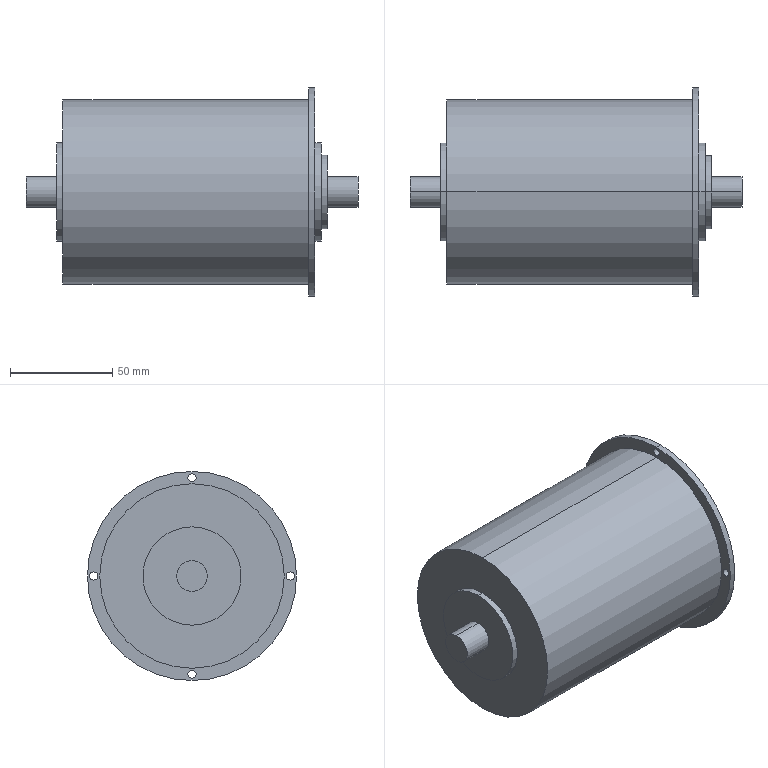Part | NX | features BREP 1 | 1 solid | 30 faces | box 162 x 102 x 102 mm | volume 806982 mm3 | cylinder 22 | plane 8 | commonest cylinder face diameters 4 x8 15 x4 48 x4 36 x2 90 x2 102 x2
STEP:
#1=CARTESIAN_POINT('',(141.,0.,-46.));
#2=VERTEX_POINT('',#1);
#3=CARTESIAN_POINT('',(141.,0.,-50.));
#4=VERTEX_POINT('',#3);
#5=CARTESIAN_POINT('',(141.,0.,-48.));
#6=DIRECTION('',(1.,0.,0.));
#7=DIRECTION('',(0.,0.,1.));
#8=AXIS2_PLACEMENT_3D('',#5,#6,#7);
#9=CIRCLE('',#8,2.);
#10=EDGE_CURVE('',#2,#4,#9,.T.);
#11=ORIENTED_EDGE('',*,*,#10,.T.);
#12=CARTESIAN_POINT('',(138.,0.,-50.));
#13=VERTEX_POINT('',#12);
#14=CARTESIAN_POINT('',(162.001,0.,-50.));
#15=DIRECTION('',(-1.,0.,0.));
#16=VECTOR('',#15,1000.);
#17=LINE('',#14,#16);
#18=EDGE_CURVE('',#4,#13,#17,.T.);
#19=ORIENTED_EDGE('',*,*,#18,.T.);
#20=CARTESIAN_POINT('',(138.,0.,-46.));
#21=VERTEX_POINT('',#20);
#22=CARTESIAN_POINT('',(138.,0.,-48.));
#23=DIRECTION('',(-1.,0.,0.));
#24=DIRECTION('',(0.,0.,1.));
#25=AXIS2_PLACEMENT_3D('',#22,#23,#24);
#26=CIRCLE('',#25,2.);
#27=EDGE_CURVE('',#13,#21,#26,.T.);
#28=ORIENTED_EDGE('',*,*,#27,.T.);
#29=CARTESIAN_POINT('',(162.001,0.,-46.));
#30=DIRECTION('',(-1.,0.,0.));
#31=VECTOR('',#30,1000.);
#32=LINE('',#29,#31);
#33=EDGE_CURVE('',#2,#21,#32,.T.);
#34=ORIENTED_EDGE('',*,*,#33,.F.);
#35=EDGE_LOOP('',(#11,#19,#28,#34));
#36=FACE_BOUND('',#35,.T.);
#37=CARTESIAN_POINT('',(162.001,0.,-48.));
#38=DIRECTION('',(-1.,0.,0.));
#39=DIRECTION('',(0.,0.,-1.));
#40=AXIS2_PLACEMENT_3D('',#37,#38,#39);
#41=CYLINDRICAL_SURFACE('',#40,2.);
#42=ADVANCED_FACE('',(#36),#41,.F.);
#43=CARTESIAN_POINT('',(141.,-48.,2.));
#44=VERTEX_POINT('',#43);
#45=CARTESIAN_POINT('',(141.,-48.,-2.));
#46=VERTEX_POINT('',#45);
#47=CARTESIAN_POINT('',(141.,-48.,0.));
#48=DIRECTION('',(1.,0.,0.));
#49=DIRECTION('',(0.,0.,1.));
#50=AXIS2_PLACEMENT_3D('',#47,#48,#49);
#51=CIRCLE('',#50,2.);
#52=EDGE_CURVE('',#44,#46,#51,.T.);
#53=ORIENTED_EDGE('',*,*,#52,.T.);
#54=CARTESIAN_POINT('',(138.,-48.,-2.));
#55=VERTEX_POINT('',#54);
#56=CARTESIAN_POINT('',(162.001,-48.,-2.));
#57=DIRECTION('',(-1.,0.,0.));
#58=VECTOR('',#57,1000.);
#59=LINE('',#56,#58);
#60=EDGE_CURVE('',#46,#55,#59,.T.);
#61=ORIENTED_EDGE('',*,*,#60,.T.);
#62=CARTESIAN_POINT('',(138.,-48.,2.));
#63=VERTEX_POINT('',#62);
#64=CARTESIAN_POINT('',(138.,-48.,0.));
#65=DIRECTION('',(-1.,0.,0.));
#66=DIRECTION('',(0.,0.,1.));
#67=AXIS2_PLACEMENT_3D('',#64,#65,#66);
#68=CIRCLE('',#67,2.);
#69=EDGE_CURVE('',#55,#63,#68,.T.);
#70=ORIENTED_EDGE('',*,*,#69,.T.);
#71=CARTESIAN_POINT('',(162.001,-48.,2.));
#72=DIRECTION('',(-1.,0.,0.));
#73=VECTOR('',#72,1000.);
#74=LINE('',#71,#73);
#75=EDGE_CURVE('',#44,#63,#74,.T.);
#76=ORIENTED_EDGE('',*,*,#75,.F.);
#77=EDGE_LOOP('',(#53,#61,#70,#76));
#78=FACE_BOUND('',#77,.T.);
#79=CARTESIAN_POINT('',(162.001,-48.,0.));
#80=DIRECTION('',(-1.,0.,0.));
#81=DIRECTION('',(0.,0.,-1.));
#82=AXIS2_PLACEMENT_3D('',#79,#80,#81);
#83=CYLINDRICAL_SURFACE('',#82,2.);
#84=ADVANCED_FACE('',(#78),#83,.F.);
#85=CARTESIAN_POINT('',(141.,0.,50.));
#86=VERTEX_POINT('',#85);
#87=CARTESIAN_POINT('',(141.,0.,46.));
#88=VERTEX_POINT('',#87);
#89=CARTESIAN_POINT('',(141.,0.,48.));
#90=DIRECTION('',(1.,0.,0.));
#91=DIRECTION('',(0.,0.,1.));
#92=AXIS2_PLACEMENT_3D('',#89,#90,#91);
#93=CIRCLE('',#92,2.);
#94=EDGE_CURVE('',#86,#88,#93,.T.);
#95=ORIENTED_EDGE('',*,*,#94,.T.);
#96=CARTESIAN_POINT('',(138.,0.,46.));
#97=VERTEX_POINT('',#96);
#98=CARTESIAN_POINT('',(162.001,0.,46.));
#99=DIRECTION('',(-1.,0.,0.));
#100=VECTOR('',#99,1000.);
#101=LINE('',#98,#100);
#102=EDGE_CURVE('',#88,#97,#101,.T.);
#103=ORIENTED_EDGE('',*,*,#102,.T.);
#104=CARTESIAN_POINT('',(138.,0.,50.));
#105=VERTEX_POINT('',#104);
#106=CARTESIAN_POINT('',(138.,0.,48.));
#107=DIRECTION('',(-1.,0.,0.));
#108=DIRECTION('',(0.,0.,1.));
#109=AXIS2_PLACEMENT_3D('',#106,#107,#108);
#110=CIRCLE('',#109,2.);
#111=EDGE_CURVE('',#97,#105,#110,.T.);
#112=ORIENTED_EDGE('',*,*,#111,.T.);
#113=CARTESIAN_POINT('',(162.001,0.,50.));
#114=DIRECTION('',(-1.,0.,0.));
#115=VECTOR('',#114,1000.);
#116=LINE('',#113,#115);
#117=EDGE_CURVE('',#86,#105,#116,.T.);
#118=ORIENTED_EDGE('',*,*,#117,.F.);
#119=EDGE_LOOP('',(#95,#103,#112,#118));
#120=FACE_BOUND('',#119,.T.);
#121=CARTESIAN_POINT('',(162.001,0.,48.));
#122=DIRECTION('',(-1.,0.,0.));
#123=DIRECTION('',(0.,0.,-1.));
#124=AXIS2_PLACEMENT_3D('',#121,#122,#123);
#125=CYLINDRICAL_SURFACE('',#124,2.);
#126=ADVANCED_FACE('',(#120),#125,.F.);
#127=CARTESIAN_POINT('',(141.,48.,2.));
#128=VERTEX_POINT('',#127);
#129=CARTESIAN_POINT('',(141.,48.,-2.));
#130=VERTEX_POINT('',#129);
#131=CARTESIAN_POINT('',(141.,48.,0.));
#132=DIRECTION('',(1.,0.,0.));
#133=DIRECTION('',(0.,0.,1.));
#134=AXIS2_PLACEMENT_3D('',#131,#132,#133);
#135=CIRCLE('',#134,2.);
#136=EDGE_CURVE('',#128,#130,#135,.T.);
#137=ORIENTED_EDGE('',*,*,#136,.T.);
#138=CARTESIAN_POINT('',(138.,48.,-2.));
#139=VERTEX_POINT('',#138);
#140=CARTESIAN_POINT('',(162.001,48.,-2.));
#141=DIRECTION('',(-1.,0.,0.));
#142=VECTOR('',#141,1000.);
#143=LINE('',#140,#142);
#144=EDGE_CURVE('',#130,#139,#143,.T.);
#145=ORIENTED_EDGE('',*,*,#144,.T.);
#146=CARTESIAN_POINT('',(138.,48.,2.));
#147=VERTEX_POINT('',#146);
#148=CARTESIAN_POINT('',(138.,48.,0.));
#149=DIRECTION('',(-1.,0.,0.));
#150=DIRECTION('',(0.,0.,1.));
#151=AXIS2_PLACEMENT_3D('',#148,#149,#150);
#152=CIRCLE('',#151,2.);
#153=EDGE_CURVE('',#139,#147,#152,.T.);
#154=ORIENTED_EDGE('',*,*,#153,.T.);
#155=CARTESIAN_POINT('',(162.001,48.,2.));
#156=DIRECTION('',(-1.,0.,0.));
#157=VECTOR('',#156,1000.);
#158=LINE('',#155,#157);
#159=EDGE_CURVE('',#128,#147,#158,.T.);
#160=ORIENTED_EDGE('',*,*,#159,.F.);
#161=EDGE_LOOP('',(#137,#145,#154,#160));
#162=FACE_BOUND('',#161,.T.);
#163=CARTESIAN_POINT('',(162.001,48.,0.));
#164=DIRECTION('',(-1.,0.,0.));
#165=DIRECTION('',(0.,0.,-1.));
#166=AXIS2_PLACEMENT_3D('',#163,#164,#165);
#167=CYLINDRICAL_SURFACE('',#166,2.);
#168=ADVANCED_FACE('',(#162),#167,.F.);
#169=CARTESIAN_POINT('',(162.,0.,7.5));
#170=VERTEX_POINT('',#169);
#171=CARTESIAN_POINT('',(162.,0.,-7.5));
#172=VERTEX_POINT('',#171);
#173=CARTESIAN_POINT('',(162.,0.,0.));
#174=DIRECTION('',(-1.,0.,0.));
#175=DIRECTION('',(0.,0.,1.));
#176=AXIS2_PLACEMENT_3D('',#173,#174,#175);
#177=CIRCLE('',#176,7.5);
#178=EDGE_CURVE('',#170,#172,#177,.T.);
#179=ORIENTED_EDGE('',*,*,#178,.T.);
#180=CARTESIAN_POINT('',(147.,0.,-7.5));
#181=VERTEX_POINT('',#180);
#182=CARTESIAN_POINT('',(0.,0.,-7.5));
#183=DIRECTION('',(-1.,0.,0.));
#184=VECTOR('',#183,1000.);
#185=LINE('',#182,#184);
#186=EDGE_CURVE('',#172,#181,#185,.T.);
#187=ORIENTED_EDGE('',*,*,#186,.T.);
#188=CARTESIAN_POINT('',(147.,0.,7.5));
#189=VERTEX_POINT('',#188);
#190=CARTESIAN_POINT('',(147.,0.,0.));
#191=DIRECTION('',(-1.,0.,0.));
#192=DIRECTION('',(0.,0.,1.));
#193=AXIS2_PLACEMENT_3D('',#190,#191,#192);
#194=CIRCLE('',#193,7.5);
#195=EDGE_CURVE('',#189,#181,#194,.T.);
#196=ORIENTED_EDGE('',*,*,#195,.F.);
#197=CARTESIAN_POINT('',(0.,0.,7.5));
#198=DIRECTION('',(-1.,0.,0.));
#199=VECTOR('',#198,1000.);
#200=LINE('',#197,#199);
#201=EDGE_CURVE('',#170,#189,#200,.T.);
#202=ORIENTED_EDGE('',*,*,#201,.F.);
#203=EDGE_LOOP('',(#179,#187,#196,#202));
#204=FACE_BOUND('',#203,.T.);
#205=CARTESIAN_POINT('',(0.,0.,0.));
#206=DIRECTION('',(-1.,0.,0.));
#207=DIRECTION('',(0.,0.,-1.));
#208=AXIS2_PLACEMENT_3D('',#205,#206,#207);
#209=CYLINDRICAL_SURFACE('',#208,7.5);
#210=ADVANCED_FACE('',(#204),#209,.T.);
#211=CARTESIAN_POINT('',(147.,0.,18.));
#212=VERTEX_POINT('',#211);
#213=CARTESIAN_POINT('',(147.,0.,-18.));
#214=VERTEX_POINT('',#213);
#215=CARTESIAN_POINT('',(147.,0.,0.));
#216=DIRECTION('',(-1.,0.,0.));
#217=DIRECTION('',(0.,0.,1.));
#218=AXIS2_PLACEMENT_3D('',#215,#216,#217);
#219=CIRCLE('',#218,18.);
#220=EDGE_CURVE('',#212,#214,#219,.T.);
#221=ORIENTED_EDGE('',*,*,#220,.T.);
#222=CARTESIAN_POINT('',(144.,0.,-18.));
#223=VERTEX_POINT('',#222);
#224=CARTESIAN_POINT('',(0.,0.,-18.));
#225=DIRECTION('',(-1.,0.,0.));
#226=VECTOR('',#225,1000.);
#227=LINE('',#224,#226);
#228=EDGE_CURVE('',#214,#223,#227,.T.);
#229=ORIENTED_EDGE('',*,*,#228,.T.);
#230=CARTESIAN_POINT('',(144.,0.,18.));
#231=VERTEX_POINT('',#230);
#232=CARTESIAN_POINT('',(144.,0.,0.));
#233=DIRECTION('',(-1.,0.,0.));
#234=DIRECTION('',(0.,0.,1.));
#235=AXIS2_PLACEMENT_3D('',#232,#233,#234);
#236=CIRCLE('',#235,18.);
#237=EDGE_CURVE('',#231,#223,#236,.T.);
#238=ORIENTED_EDGE('',*,*,#237,.F.);
#239=CARTESIAN_POINT('',(0.,0.,18.));
#240=DIRECTION('',(-1.,0.,0.));
#241=VECTOR('',#240,1000.);
#242=LINE('',#239,#241);
#243=EDGE_CURVE('',#212,#231,#242,.T.);
#244=ORIENTED_EDGE('',*,*,#243,.F.);
#245=EDGE_LOOP('',(#221,#229,#238,#244));
#246=FACE_BOUND('',#245,.T.);
#247=CARTESIAN_POINT('',(0.,0.,0.));
#248=DIRECTION('',(-1.,0.,0.));
#249=DIRECTION('',(0.,0.,-1.));
#250=AXIS2_PLACEMENT_3D('',#247,#248,#249);
#251=CYLINDRICAL_SURFACE('',#250,18.);
#252=ADVANCED_FACE('',(#246),#251,.T.);
#253=CARTESIAN_POINT('',(144.,0.,24.));
#254=VERTEX_POINT('',#253);
#255=CARTESIAN_POINT('',(144.,0.,-24.));
#256=VERTEX_POINT('',#255);
#257=CARTESIAN_POINT('',(144.,0.,0.));
#258=DIRECTION('',(-1.,0.,0.));
#259=DIRECTION('',(0.,0.,1.));
#260=AXIS2_PLACEMENT_3D('',#257,#258,#259);
#261=CIRCLE('',#260,24.);
#262=EDGE_CURVE('',#254,#256,#261,.T.);
#263=ORIENTED_EDGE('',*,*,#262,.T.);
#264=CARTESIAN_POINT('',(141.,0.,-24.));
#265=VERTEX_POINT('',#264);
#266=CARTESIAN_POINT('',(0.,0.,-24.));
#267=DIRECTION('',(-1.,0.,0.));
#268=VECTOR('',#267,1000.);
#269=LINE('',#266,#268);
#270=EDGE_CURVE('',#256,#265,#269,.T.);
#271=ORIENTED_EDGE('',*,*,#270,.T.);
#272=CARTESIAN_POINT('',(141.,0.,24.));
#273=VERTEX_POINT('',#272);
#274=CARTESIAN_POINT('',(141.,0.,0.));
#275=DIRECTION('',(-1.,0.,0.));
#276=DIRECTION('',(0.,0.,1.));
#277=AXIS2_PLACEMENT_3D('',#274,#275,#276);
#278=CIRCLE('',#277,24.);
#279=EDGE_CURVE('',#273,#265,#278,.T.);
#280=ORIENTED_EDGE('',*,*,#279,.F.);
#281=CARTESIAN_POINT('',(0.,0.,24.));
#282=DIRECTION('',(-1.,0.,0.));
#283=VECTOR('',#282,1000.);
#284=LINE('',#281,#283);
#285=EDGE_CURVE('',#254,#273,#284,.T.);
#286=ORIENTED_EDGE('',*,*,#285,.F.);
#287=EDGE_LOOP('',(#263,#271,#280,#286));
#288=FACE_BOUND('',#287,.T.);
#289=CARTESIAN_POINT('',(0.,0.,0.));
#290=DIRECTION('',(-1.,0.,0.));
#291=DIRECTION('',(0.,0.,-1.));
#292=AXIS2_PLACEMENT_3D('',#289,#290,#291);
#293=CYLINDRICAL_SURFACE('',#292,24.);
#294=ADVANCED_FACE('',(#288),#293,.T.);
#295=CARTESIAN_POINT('',(141.,0.,51.));
#296=VERTEX_POINT('',#295);
#297=CARTESIAN_POINT('',(141.,0.,-51.));
#298=VERTEX_POINT('',#297);
#299=CARTESIAN_POINT('',(141.,0.,0.));
#300=DIRECTION('',(-1.,0.,0.));
#301=DIRECTION('',(0.,0.,1.));
#302=AXIS2_PLACEMENT_3D('',#299,#300,#301);
#303=CIRCLE('',#302,51.);
#304=EDGE_CURVE('',#296,#298,#303,.T.);
#305=ORIENTED_EDGE('',*,*,#304,.T.);
#306=CARTESIAN_POINT('',(138.,0.,-51.));
#307=VERTEX_POINT('',#306);
#308=CARTESIAN_POINT('',(0.,0.,-51.));
#309=DIRECTION('',(-1.,0.,0.));
#310=VECTOR('',#309,1000.);
#311=LINE('',#308,#310);
#312=EDGE_CURVE('',#298,#307,#311,.T.);
#313=ORIENTED_EDGE('',*,*,#312,.T.);
#314=CARTESIAN_POINT('',(138.,0.,51.));
#315=VERTEX_POINT('',#314);
#316=CARTESIAN_POINT('',(138.,0.,0.));
#317=DIRECTION('',(-1.,0.,0.));
#318=DIRECTION('',(0.,0.,1.));
#319=AXIS2_PLACEMENT_3D('',#316,#317,#318);
#320=CIRCLE('',#319,51.);
#321=EDGE_CURVE('',#315,#307,#320,.T.);
#322=ORIENTED_EDGE('',*,*,#321,.F.);
#323=CARTESIAN_POINT('',(0.,0.,51.));
#324=DIRECTION('',(-1.,0.,0.));
#325=VECTOR('',#324,1000.);
#326=LINE('',#323,#325);
#327=EDGE_CURVE('',#296,#315,#326,.T.);
#328=ORIENTED_EDGE('',*,*,#327,.F.);
#329=EDGE_LOOP('',(#305,#313,#322,#328));
#330=FACE_BOUND('',#329,.T.);
#331=CARTESIAN_POINT('',(0.,0.,0.));
#332=DIRECTION('',(-1.,0.,0.));
#333=DIRECTION('',(0.,0.,-1.));
#334=AXIS2_PLACEMENT_3D('',#331,#332,#333);
#335=CYLINDRICAL_SURFACE('',#334,51.);
#336=ADVANCED_FACE('',(#330),#335,.T.);
#337=CARTESIAN_POINT('',(138.,0.,45.));
#338=VERTEX_POINT('',#337);
#339=CARTESIAN_POINT('',(138.,0.,-45.));
#340=VERTEX_POINT('',#339);
#341=CARTESIAN_POINT('',(138.,0.,0.));
#342=DIRECTION('',(-1.,0.,0.));
#343=DIRECTION('',(0.,0.,1.));
#344=AXIS2_PLACEMENT_3D('',#341,#342,#343);
#345=CIRCLE('',#344,45.);
#346=EDGE_CURVE('',#338,#340,#345,.T.);
#347=ORIENTED_EDGE('',*,*,#346,.T.);
#348=CARTESIAN_POINT('',(18.,0.,-45.));
#349=VERTEX_POINT('',#348);
#350=CARTESIAN_POINT('',(0.,0.,-45.));
#351=DIRECTION('',(-1.,0.,0.));
#352=VECTOR('',#351,1000.);
#353=LINE('',#350,#352);
#354=EDGE_CURVE('',#340,#349,#353,.T.);
#355=ORIENTED_EDGE('',*,*,#354,.T.);
#356=CARTESIAN_POINT('',(18.,0.,45.));
#357=VERTEX_POINT('',#356);
#358=CARTESIAN_POINT('',(18.,0.,0.));
#359=DIRECTION('',(-1.,0.,0.));
#360=DIRECTION('',(0.,0.,1.));
#361=AXIS2_PLACEMENT_3D('',#358,#359,#360);
#362=CIRCLE('',#361,45.);
#363=EDGE_CURVE('',#357,#349,#362,.T.);
#364=ORIENTED_EDGE('',*,*,#363,.F.);
#365=CARTESIAN_POINT('',(0.,0.,45.));
#366=DIRECTION('',(-1.,0.,0.));
#367=VECTOR('',#366,1000.);
#368=LINE('',#365,#367);
#369=EDGE_CURVE('',#338,#357,#368,.T.);
#370=ORIENTED_EDGE('',*,*,#369,.F.);
#371=EDGE_LOOP('',(#347,#355,#364,#370));
#372=FACE_BOUND('',#371,.T.);
#373=CARTESIAN_POINT('',(0.,0.,0.));
#374=DIRECTION('',(-1.,0.,0.));
#375=DIRECTION('',(0.,0.,-1.));
#376=AXIS2_PLACEMENT_3D('',#373,#374,#375);
#377=CYLINDRICAL_SURFACE('',#376,45.);
#378=ADVANCED_FACE('',(#372),#377,.T.);
#379=CARTESIAN_POINT('',(18.,0.,24.));
#380=VERTEX_POINT('',#379);
#381=CARTESIAN_POINT('',(18.,0.,-24.));
#382=VERTEX_POINT('',#381);
#383=CARTESIAN_POINT('',(18.,0.,0.));
#384=DIRECTION('',(-1.,0.,0.));
#385=DIRECTION('',(0.,0.,1.));
#386=AXIS2_PLACEMENT_3D('',#383,#384,#385);
#387=CIRCLE('',#386,24.);
#388=EDGE_CURVE('',#380,#382,#387,.T.);
#389=ORIENTED_EDGE('',*,*,#388,.T.);
#390=CARTESIAN_POINT('',(15.,0.,-24.));
#391=VERTEX_POINT('',#390);
#392=CARTESIAN_POINT('',(0.,0.,-24.));
#393=DIRECTION('',(-1.,0.,0.));
#394=VECTOR('',#393,1000.);
#395=LINE('',#392,#394);
#396=EDGE_CURVE('',#382,#391,#395,.T.);
#397=ORIENTED_EDGE('',*,*,#396,.T.);
#398=CARTESIAN_POINT('',(15.,0.,24.));
#399=VERTEX_POINT('',#398);
#400=CARTESIAN_POINT('',(15.,0.,0.));
#401=DIRECTION('',(-1.,0.,0.));
#402=DIRECTION('',(0.,0.,1.));
#403=AXIS2_PLACEMENT_3D('',#400,#401,#402);
#404=CIRCLE('',#403,24.);
#405=EDGE_CURVE('',#399,#391,#404,.T.);
#406=ORIENTED_EDGE('',*,*,#405,.F.);
#407=CARTESIAN_POINT('',(0.,0.,24.));
#408=DIRECTION('',(-1.,0.,0.));
#409=VECTOR('',#408,1000.);
#410=LINE('',#407,#409);
#411=EDGE_CURVE('',#380,#399,#410,.T.);
#412=ORIENTED_EDGE('',*,*,#411,.F.);
#413=EDGE_LOOP('',(#389,#397,#406,#412));
#414=FACE_BOUND('',#413,.T.);
#415=CARTESIAN_POINT('',(0.,0.,0.));
#416=DIRECTION('',(-1.,0.,0.));
#417=DIRECTION('',(0.,0.,-1.));
#418=AXIS2_PLACEMENT_3D('',#415,#416,#417);
#419=CYLINDRICAL_SURFACE('',#418,24.);
#420=ADVANCED_FACE('',(#414),#419,.T.);
#421=CARTESIAN_POINT('',(15.,0.,7.5));
#422=VERTEX_POINT('',#421);
#423=CARTESIAN_POINT('',(15.,0.,-7.5));
#424=VERTEX_POINT('',#423);
#425=CARTESIAN_POINT('',(15.,0.,0.));
#426=DIRECTION('',(-1.,0.,0.));
#427=DIRECTION('',(0.,0.,1.));
#428=AXIS2_PLACEMENT_3D('',#425,#426,#427);
#429=CIRCLE('',#428,7.5);
#430=EDGE_CURVE('',#422,#424,#429,.T.);
#431=ORIENTED_EDGE('',*,*,#430,.T.);
#432=CARTESIAN_POINT('',(0.,0.,-7.5));
#433=VERTEX_POINT('',#432);
#434=CARTESIAN_POINT('',(0.,0.,-7.5));
#435=DIRECTION('',(-1.,0.,0.));
#436=VECTOR('',#435,1000.);
#437=LINE('',#434,#436);
#438=EDGE_CURVE('',#424,#433,#437,.T.);
#439=ORIENTED_EDGE('',*,*,#438,.T.);
#440=CARTESIAN_POINT('',(0.,0.,7.5));
#441=VERTEX_POINT('',#440);
#442=CARTESIAN_POINT('',(0.,0.,0.));
#443=DIRECTION('',(-1.,0.,0.));
#444=DIRECTION('',(0.,0.,1.));
#445=AXIS2_PLACEMENT_3D('',#442,#443,#444);
#446=CIRCLE('',#445,7.5);
#447=EDGE_CURVE('',#441,#433,#446,.T.);
#448=ORIENTED_EDGE('',*,*,#447,.F.);
#449=CARTESIAN_POINT('',(0.,0.,7.5));
#450=DIRECTION('',(-1.,0.,0.));
#451=VECTOR('',#450,1000.);
#452=LINE('',#449,#451);
#453=EDGE_CURVE('',#422,#441,#452,.T.);
#454=ORIENTED_EDGE('',*,*,#453,.F.);
#455=EDGE_LOOP('',(#431,#439,#448,#454));
#456=FACE_BOUND('',#455,.T.);
#457=CARTESIAN_POINT('',(0.,0.,0.));
#458=DIRECTION('',(-1.,0.,0.));
#459=DIRECTION('',(0.,0.,-1.));
#460=AXIS2_PLACEMENT_3D('',#457,#458,#459);
#461=CYLINDRICAL_SURFACE('',#460,7.5);
#462=ADVANCED_FACE('',(#456),#461,.T.);
#463=ORIENTED_EDGE('',*,*,#447,.T.);
#464=CARTESIAN_POINT('',(0.,0.,0.));
#465=DIRECTION('',(-1.,0.,0.));
#466=DIRECTION('',(0.,0.,1.));
#467=AXIS2_PLACEMENT_3D('',#464,#465,#466);
#468=CIRCLE('',#467,7.5);
#469=EDGE_CURVE('',#433,#441,#468,.T.);
#470=ORIENTED_EDGE('',*,*,#469,.T.);
#471=EDGE_LOOP('',(#463,#470));
#472=FACE_BOUND('',#471,.T.);
#473=CARTESIAN_POINT('',(0.,0.,0.));
#474=DIRECTION('',(1.,0.,0.));
#475=DIRECTION('',(0.,-1.,0.));
#476=AXIS2_PLACEMENT_3D('',#473,#474,#475);
#477=PLANE('',#476);
#478=ADVANCED_FACE('',(#472),#477,.F.);
#479=ORIENTED_EDGE('',*,*,#438,.F.);
#480=CARTESIAN_POINT('',(15.,0.,0.));
#481=DIRECTION('',(-1.,0.,0.));
#482=DIRECTION('',(0.,0.,1.));
#483=AXIS2_PLACEMENT_3D('',#480,#481,#482);
#484=CIRCLE('',#483,7.5);
#485=EDGE_CURVE('',#424,#422,#484,.T.);
#486=ORIENTED_EDGE('',*,*,#485,.T.);
#487=ORIENTED_EDGE('',*,*,#453,.T.);
#488=ORIENTED_EDGE('',*,*,#469,.F.);
#489=EDGE_LOOP('',(#479,#486,#487,#488));
#490=FACE_BOUND('',#489,.T.);
#491=CARTESIAN_POINT('',(0.,0.,0.));
#492=DIRECTION('',(-1.,0.,0.));
#493=DIRECTION('',(0.,0.,-1.));
#494=AXIS2_PLACEMENT_3D('',#491,#492,#493);
#495=CYLINDRICAL_SURFACE('',#494,7.5);
#496=ADVANCED_FACE('',(#490),#495,.T.);
#497=ORIENTED_EDGE('',*,*,#405,.T.);
#498=CARTESIAN_POINT('',(15.,0.,0.));
#499=DIRECTION('',(-1.,0.,0.));
#500=DIRECTION('',(0.,0.,1.));
#501=AXIS2_PLACEMENT_3D('',#498,#499,#500);
#502=CIRCLE('',#501,24.);
#503=EDGE_CURVE('',#391,#399,#502,.T.);
#504=ORIENTED_EDGE('',*,*,#503,.T.);
#505=EDGE_LOOP('',(#497,#504));
#506=FACE_BOUND('',#505,.T.);
#507=ORIENTED_EDGE('',*,*,#430,.F.);
#508=ORIENTED_EDGE('',*,*,#485,.F.);
#509=EDGE_LOOP('',(#507,#508));
#510=FACE_BOUND('',#509,.T.);
#511=CARTESIAN_POINT('',(15.,7.5,0.));
#512=DIRECTION('',(1.,0.,0.));
#513=DIRECTION('',(0.,-1.,0.));
#514=AXIS2_PLACEMENT_3D('',#511,#512,#513);
#515=PLANE('',#514);
#516=ADVANCED_FACE('',(#506,#510),#515,.F.);
#517=ORIENTED_EDGE('',*,*,#396,.F.);
#518=CARTESIAN_POINT('',(18.,0.,0.));
#519=DIRECTION('',(-1.,0.,0.));
#520=DIRECTION('',(0.,0.,1.));
#521=AXIS2_PLACEMENT_3D('',#518,#519,#520);
#522=CIRCLE('',#521,24.);
#523=EDGE_CURVE('',#382,#380,#522,.T.);
#524=ORIENTED_EDGE('',*,*,#523,.T.);
#525=ORIENTED_EDGE('',*,*,#411,.T.);
#526=ORIENTED_EDGE('',*,*,#503,.F.);
#527=EDGE_LOOP('',(#517,#524,#525,#526));
#528=FACE_BOUND('',#527,.T.);
#529=CARTESIAN_POINT('',(0.,0.,0.));
#530=DIRECTION('',(-1.,0.,0.));
#531=DIRECTION('',(0.,0.,-1.));
#532=AXIS2_PLACEMENT_3D('',#529,#530,#531);
#533=CYLINDRICAL_SURFACE('',#532,24.);
#534=ADVANCED_FACE('',(#528),#533,.T.);
#535=ORIENTED_EDGE('',*,*,#363,.T.);
#536=CARTESIAN_POINT('',(18.,0.,0.));
#537=DIRECTION('',(-1.,0.,0.));
#538=DIRECTION('',(0.,0.,1.));
#539=AXIS2_PLACEMENT_3D('',#536,#537,#538);
#540=CIRCLE('',#539,45.);
#541=EDGE_CURVE('',#349,#357,#540,.T.);
#542=ORIENTED_EDGE('',*,*,#541,.T.);
#543=EDGE_LOOP('',(#535,#542));
#544=FACE_BOUND('',#543,.T.);
#545=ORIENTED_EDGE('',*,*,#388,.F.);
#546=ORIENTED_EDGE('',*,*,#523,.F.);
#547=EDGE_LOOP('',(#545,#546));
#548=FACE_BOUND('',#547,.T.);
#549=CARTESIAN_POINT('',(18.,24.,0.));
#550=DIRECTION('',(1.,0.,0.));
#551=DIRECTION('',(0.,-1.,0.));
#552=AXIS2_PLACEMENT_3D('',#549,#550,#551);
#553=PLANE('',#552);
#554=ADVANCED_FACE('',(#544,#548),#553,.F.);
#555=ORIENTED_EDGE('',*,*,#354,.F.);
#556=CARTESIAN_POINT('',(138.,0.,0.));
#557=DIRECTION('',(-1.,0.,0.));
#558=DIRECTION('',(0.,0.,1.));
#559=AXIS2_PLACEMENT_3D('',#556,#557,#558);
#560=CIRCLE('',#559,45.);
#561=EDGE_CURVE('',#340,#338,#560,.T.);
#562=ORIENTED_EDGE('',*,*,#561,.T.);
#563=ORIENTED_EDGE('',*,*,#369,.T.);
#564=ORIENTED_EDGE('',*,*,#541,.F.);
#565=EDGE_LOOP('',(#555,#562,#563,#564));
#566=FACE_BOUND('',#565,.T.);
#567=CARTESIAN_POINT('',(0.,0.,0.));
#568=DIRECTION('',(-1.,0.,0.));
#569=DIRECTION('',(0.,0.,-1.));
#570=AXIS2_PLACEMENT_3D('',#567,#568,#569);
#571=CYLINDRICAL_SURFACE('',#570,45.);
#572=ADVANCED_FACE('',(#566),#571,.T.);
#573=ORIENTED_EDGE('',*,*,#321,.T.);
#574=CARTESIAN_POINT('',(138.,0.,0.));
#575=DIRECTION('',(-1.,0.,0.));
#576=DIRECTION('',(0.,0.,1.));
#577=AXIS2_PLACEMENT_3D('',#574,#575,#576);
#578=CIRCLE('',#577,51.);
#579=EDGE_CURVE('',#307,#315,#578,.T.);
#580=ORIENTED_EDGE('',*,*,#579,.T.);
#581=EDGE_LOOP('',(#573,#580));
#582=FACE_BOUND('',#581,.T.);
#583=CARTESIAN_POINT('',(138.,0.,-48.));
#584=DIRECTION('',(-1.,0.,0.));
#585=DIRECTION('',(0.,0.,1.));
#586=AXIS2_PLACEMENT_3D('',#583,#584,#585);
#587=CIRCLE('',#586,2.);
#588=EDGE_CURVE('',#21,#13,#587,.T.);
#589=ORIENTED_EDGE('',*,*,#588,.F.);
#590=ORIENTED_EDGE('',*,*,#27,.F.);
#591=EDGE_LOOP('',(#589,#590));
#592=FACE_BOUND('',#591,.T.);
#593=CARTESIAN_POINT('',(138.,-48.,0.));
#594=DIRECTION('',(-1.,0.,0.));
#595=DIRECTION('',(0.,0.,1.));
#596=AXIS2_PLACEMENT_3D('',#593,#594,#595);
#597=CIRCLE('',#596,2.);
#598=EDGE_CURVE('',#63,#55,#597,.T.);
#599=ORIENTED_EDGE('',*,*,#598,.F.);
#600=ORIENTED_EDGE('',*,*,#69,.F.);
#601=EDGE_LOOP('',(#599,#600));
#602=FACE_BOUND('',#601,.T.);
#603=CARTESIAN_POINT('',(138.,0.,48.));
#604=DIRECTION('',(-1.,0.,0.));
#605=DIRECTION('',(0.,0.,1.));
#606=AXIS2_PLACEMENT_3D('',#603,#604,#605);
#607=CIRCLE('',#606,2.);
#608=EDGE_CURVE('',#105,#97,#607,.T.);
#609=ORIENTED_EDGE('',*,*,#608,.F.);
#610=ORIENTED_EDGE('',*,*,#111,.F.);
#611=EDGE_LOOP('',(#609,#610));
#612=FACE_BOUND('',#611,.T.);
#613=CARTESIAN_POINT('',(138.,48.,0.));
#614=DIRECTION('',(-1.,0.,0.));
#615=DIRECTION('',(0.,0.,1.));
#616=AXIS2_PLACEMENT_3D('',#613,#614,#615);
#617=CIRCLE('',#616,2.);
#618=EDGE_CURVE('',#147,#139,#617,.T.);
#619=ORIENTED_EDGE('',*,*,#618,.F.);
#620=ORIENTED_EDGE('',*,*,#153,.F.);
#621=EDGE_LOOP('',(#619,#620));
#622=FACE_BOUND('',#621,.T.);
#623=ORIENTED_EDGE('',*,*,#346,.F.);
#624=ORIENTED_EDGE('',*,*,#561,.F.);
#625=EDGE_LOOP('',(#623,#624));
#626=FACE_BOUND('',#625,.T.);
#627=CARTESIAN_POINT('',(138.,51.,0.));
#628=DIRECTION('',(1.,0.,0.));
#629=DIRECTION('',(0.,-1.,0.));
#630=AXIS2_PLACEMENT_3D('',#627,#628,#629);
#631=PLANE('',#630);
#632=ADVANCED_FACE('',(#582,#592,#602,#612,#622,#626),#631,.F.);
#633=ORIENTED_EDGE('',*,*,#312,.F.);
#634=CARTESIAN_POINT('',(141.,0.,0.));
#635=DIRECTION('',(-1.,0.,0.));
#636=DIRECTION('',(0.,0.,1.));
#637=AXIS2_PLACEMENT_3D('',#634,#635,#636);
#638=CIRCLE('',#637,51.);
#639=EDGE_CURVE('',#298,#296,#638,.T.);
#640=ORIENTED_EDGE('',*,*,#639,.T.);
#641=ORIENTED_EDGE('',*,*,#327,.T.);
#642=ORIENTED_EDGE('',*,*,#579,.F.);
#643=EDGE_LOOP('',(#633,#640,#641,#642));
#644=FACE_BOUND('',#643,.T.);
#645=CARTESIAN_POINT('',(0.,0.,0.));
#646=DIRECTION('',(-1.,0.,0.));
#647=DIRECTION('',(0.,0.,-1.));
#648=AXIS2_PLACEMENT_3D('',#645,#646,#647);
#649=CYLINDRICAL_SURFACE('',#648,51.);
#650=ADVANCED_FACE('',(#644),#649,.T.);
#651=ORIENTED_EDGE('',*,*,#304,.F.);
#652=ORIENTED_EDGE('',*,*,#639,.F.);
#653=EDGE_LOOP('',(#651,#652));
#654=FACE_BOUND('',#653,.T.);
#655=ORIENTED_EDGE('',*,*,#10,.F.);
#656=CARTESIAN_POINT('',(141.,0.,-48.));
#657=DIRECTION('',(1.,0.,0.));
#658=DIRECTION('',(0.,0.,1.));
#659=AXIS2_PLACEMENT_3D('',#656,#657,#658);
#660=CIRCLE('',#659,2.);
#661=EDGE_CURVE('',#4,#2,#660,.T.);
#662=ORIENTED_EDGE('',*,*,#661,.F.);
#663=EDGE_LOOP('',(#655,#662));
#664=FACE_BOUND('',#663,.T.);
#665=ORIENTED_EDGE('',*,*,#52,.F.);
#666=CARTESIAN_POINT('',(141.,-48.,0.));
#667=DIRECTION('',(1.,0.,0.));
#668=DIRECTION('',(0.,0.,1.));
#669=AXIS2_PLACEMENT_3D('',#666,#667,#668);
#670=CIRCLE('',#669,2.);
#671=EDGE_CURVE('',#46,#44,#670,.T.);
#672=ORIENTED_EDGE('',*,*,#671,.F.);
#673=EDGE_LOOP('',(#665,#672));
#674=FACE_BOUND('',#673,.T.);
#675=ORIENTED_EDGE('',*,*,#94,.F.);
#676=CARTESIAN_POINT('',(141.,0.,48.));
#677=DIRECTION('',(1.,0.,0.));
#678=DIRECTION('',(0.,0.,1.));
#679=AXIS2_PLACEMENT_3D('',#676,#677,#678);
#680=CIRCLE('',#679,2.);
#681=EDGE_CURVE('',#88,#86,#680,.T.);
#682=ORIENTED_EDGE('',*,*,#681,.F.);
#683=EDGE_LOOP('',(#675,#682));
#684=FACE_BOUND('',#683,.T.);
#685=ORIENTED_EDGE('',*,*,#136,.F.);
#686=CARTESIAN_POINT('',(141.,48.,0.));
#687=DIRECTION('',(1.,0.,0.));
#688=DIRECTION('',(0.,0.,1.));
#689=AXIS2_PLACEMENT_3D('',#686,#687,#688);
#690=CIRCLE('',#689,2.);
#691=EDGE_CURVE('',#130,#128,#690,.T.);
#692=ORIENTED_EDGE('',*,*,#691,.F.);
#693=EDGE_LOOP('',(#685,#692));
#694=FACE_BOUND('',#693,.T.);
#695=ORIENTED_EDGE('',*,*,#279,.T.);
#696=CARTESIAN_POINT('',(141.,0.,0.));
#697=DIRECTION('',(-1.,0.,0.));
#698=DIRECTION('',(0.,0.,1.));
#699=AXIS2_PLACEMENT_3D('',#696,#697,#698);
#700=CIRCLE('',#699,24.);
#701=EDGE_CURVE('',#265,#273,#700,.T.);
#702=ORIENTED_EDGE('',*,*,#701,.T.);
#703=EDGE_LOOP('',(#695,#702));
#704=FACE_BOUND('',#703,.T.);
#705=CARTESIAN_POINT('',(141.,51.,0.));
#706=DIRECTION('',(-1.,0.,0.));
#707=DIRECTION('',(0.,0.,-1.));
#708=AXIS2_PLACEMENT_3D('',#705,#706,#707);
#709=PLANE('',#708);
#710=ADVANCED_FACE('',(#654,#664,#674,#684,#694,#704),#709,.F.);
#711=ORIENTED_EDGE('',*,*,#270,.F.);
#712=CARTESIAN_POINT('',(144.,0.,0.));
#713=DIRECTION('',(-1.,0.,0.));
#714=DIRECTION('',(0.,0.,1.));
#715=AXIS2_PLACEMENT_3D('',#712,#713,#714);
#716=CIRCLE('',#715,24.);
#717=EDGE_CURVE('',#256,#254,#716,.T.);
#718=ORIENTED_EDGE('',*,*,#717,.T.);
#719=ORIENTED_EDGE('',*,*,#285,.T.);
#720=ORIENTED_EDGE('',*,*,#701,.F.);
#721=EDGE_LOOP('',(#711,#718,#719,#720));
#722=FACE_BOUND('',#721,.T.);
#723=CARTESIAN_POINT('',(0.,0.,0.));
#724=DIRECTION('',(-1.,0.,0.));
#725=DIRECTION('',(0.,0.,-1.));
#726=AXIS2_PLACEMENT_3D('',#723,#724,#725);
#727=CYLINDRICAL_SURFACE('',#726,24.);
#728=ADVANCED_FACE('',(#722),#727,.T.);
#729=ORIENTED_EDGE('',*,*,#262,.F.);
#730=ORIENTED_EDGE('',*,*,#717,.F.);
#731=EDGE_LOOP('',(#729,#730));
#732=FACE_BOUND('',#731,.T.);
#733=ORIENTED_EDGE('',*,*,#237,.T.);
#734=CARTESIAN_POINT('',(144.,0.,0.));
#735=DIRECTION('',(-1.,0.,0.));
#736=DIRECTION('',(0.,0.,1.));
#737=AXIS2_PLACEMENT_3D('',#734,#735,#736);
#738=CIRCLE('',#737,18.);
#739=EDGE_CURVE('',#223,#231,#738,.T.);
#740=ORIENTED_EDGE('',*,*,#739,.T.);
#741=EDGE_LOOP('',(#733,#740));
#742=FACE_BOUND('',#741,.T.);
#743=CARTESIAN_POINT('',(144.,24.,0.));
#744=DIRECTION('',(-1.,0.,0.));
#745=DIRECTION('',(0.,0.,-1.));
#746=AXIS2_PLACEMENT_3D('',#743,#744,#745);
#747=PLANE('',#746);
#748=ADVANCED_FACE('',(#732,#742),#747,.F.);
#749=ORIENTED_EDGE('',*,*,#228,.F.);
#750=CARTESIAN_POINT('',(147.,0.,0.));
#751=DIRECTION('',(-1.,0.,0.));
#752=DIRECTION('',(0.,0.,1.));
#753=AXIS2_PLACEMENT_3D('',#750,#751,#752);
#754=CIRCLE('',#753,18.);
#755=EDGE_CURVE('',#214,#212,#754,.T.);
#756=ORIENTED_EDGE('',*,*,#755,.T.);
#757=ORIENTED_EDGE('',*,*,#243,.T.);
#758=ORIENTED_EDGE('',*,*,#739,.F.);
#759=EDGE_LOOP('',(#749,#756,#757,#758));
#760=FACE_BOUND('',#759,.T.);
#761=CARTESIAN_POINT('',(0.,0.,0.));
#762=DIRECTION('',(-1.,0.,0.));
#763=DIRECTION('',(0.,0.,-1.));
#764=AXIS2_PLACEMENT_3D('',#761,#762,#763);
#765=CYLINDRICAL_SURFACE('',#764,18.);
#766=ADVANCED_FACE('',(#760),#765,.T.);
#767=ORIENTED_EDGE('',*,*,#220,.F.);
#768=ORIENTED_EDGE('',*,*,#755,.F.);
#769=EDGE_LOOP('',(#767,#768));
#770=FACE_BOUND('',#769,.T.);
#771=ORIENTED_EDGE('',*,*,#195,.T.);
#772=CARTESIAN_POINT('',(147.,0.,0.));
#773=DIRECTION('',(-1.,0.,0.));
#774=DIRECTION('',(0.,0.,1.));
#775=AXIS2_PLACEMENT_3D('',#772,#773,#774);
#776=CIRCLE('',#775,7.5);
#777=EDGE_CURVE('',#181,#189,#776,.T.);
#778=ORIENTED_EDGE('',*,*,#777,.T.);
#779=EDGE_LOOP('',(#771,#778));
#780=FACE_BOUND('',#779,.T.);
#781=CARTESIAN_POINT('',(147.,18.,0.));
#782=DIRECTION('',(-1.,0.,0.));
#783=DIRECTION('',(0.,0.,-1.));
#784=AXIS2_PLACEMENT_3D('',#781,#782,#783);
#785=PLANE('',#784);
#786=ADVANCED_FACE('',(#770,#780),#785,.F.);
#787=ORIENTED_EDGE('',*,*,#186,.F.);
#788=CARTESIAN_POINT('',(162.,0.,0.));
#789=DIRECTION('',(-1.,0.,0.));
#790=DIRECTION('',(0.,0.,1.));
#791=AXIS2_PLACEMENT_3D('',#788,#789,#790);
#792=CIRCLE('',#791,7.5);
#793=EDGE_CURVE('',#172,#170,#792,.T.);
#794=ORIENTED_EDGE('',*,*,#793,.T.);
#795=ORIENTED_EDGE('',*,*,#201,.T.);
#796=ORIENTED_EDGE('',*,*,#777,.F.);
#797=EDGE_LOOP('',(#787,#794,#795,#796));
#798=FACE_BOUND('',#797,.T.);
#799=CARTESIAN_POINT('',(0.,0.,0.));
#800=DIRECTION('',(-1.,0.,0.));
#801=DIRECTION('',(0.,0.,-1.));
#802=AXIS2_PLACEMENT_3D('',#799,#800,#801);
#803=CYLINDRICAL_SURFACE('',#802,7.5);
#804=ADVANCED_FACE('',(#798),#803,.T.);
#805=ORIENTED_EDGE('',*,*,#178,.F.);
#806=ORIENTED_EDGE('',*,*,#793,.F.);
#807=EDGE_LOOP('',(#805,#806));
#808=FACE_BOUND('',#807,.T.);
#809=CARTESIAN_POINT('',(162.,7.5,0.));
#810=DIRECTION('',(-1.,0.,0.));
#811=DIRECTION('',(0.,0.,-1.));
#812=AXIS2_PLACEMENT_3D('',#809,#810,#811);
#813=PLANE('',#812);
#814=ADVANCED_FACE('',(#808),#813,.F.);
#815=ORIENTED_EDGE('',*,*,#144,.F.);
#816=ORIENTED_EDGE('',*,*,#691,.T.);
#817=ORIENTED_EDGE('',*,*,#159,.T.);
#818=ORIENTED_EDGE('',*,*,#618,.T.);
#819=EDGE_LOOP('',(#815,#816,#817,#818));
#820=FACE_BOUND('',#819,.T.);
#821=CARTESIAN_POINT('',(162.001,48.,0.));
#822=DIRECTION('',(-1.,0.,0.));
#823=DIRECTION('',(0.,0.,-1.));
#824=AXIS2_PLACEMENT_3D('',#821,#822,#823);
#825=CYLINDRICAL_SURFACE('',#824,2.);
#826=ADVANCED_FACE('',(#820),#825,.F.);
#827=ORIENTED_EDGE('',*,*,#102,.F.);
#828=ORIENTED_EDGE('',*,*,#681,.T.);
#829=ORIENTED_EDGE('',*,*,#117,.T.);
#830=ORIENTED_EDGE('',*,*,#608,.T.);
#831=EDGE_LOOP('',(#827,#828,#829,#830));
#832=FACE_BOUND('',#831,.T.);
#833=CARTESIAN_POINT('',(162.001,0.,48.));
#834=DIRECTION('',(-1.,0.,0.));
#835=DIRECTION('',(0.,0.,-1.));
#836=AXIS2_PLACEMENT_3D('',#833,#834,#835);
#837=CYLINDRICAL_SURFACE('',#836,2.);
#838=ADVANCED_FACE('',(#832),#837,.F.);
#839=ORIENTED_EDGE('',*,*,#60,.F.);
#840=ORIENTED_EDGE('',*,*,#671,.T.);
#841=ORIENTED_EDGE('',*,*,#75,.T.);
#842=ORIENTED_EDGE('',*,*,#598,.T.);
#843=EDGE_LOOP('',(#839,#840,#841,#842));
#844=FACE_BOUND('',#843,.T.);
#845=CARTESIAN_POINT('',(162.001,-48.,0.));
#846=DIRECTION('',(-1.,0.,0.));
#847=DIRECTION('',(0.,0.,-1.));
#848=AXIS2_PLACEMENT_3D('',#845,#846,#847);
#849=CYLINDRICAL_SURFACE('',#848,2.);
#850=ADVANCED_FACE('',(#844),#849,.F.);
#851=ORIENTED_EDGE('',*,*,#18,.F.);
#852=ORIENTED_EDGE('',*,*,#661,.T.);
#853=ORIENTED_EDGE('',*,*,#33,.T.);
#854=ORIENTED_EDGE('',*,*,#588,.T.);
#855=EDGE_LOOP('',(#851,#852,#853,#854));
#856=FACE_BOUND('',#855,.T.);
#857=CARTESIAN_POINT('',(162.001,0.,-48.));
#858=DIRECTION('',(-1.,0.,0.));
#859=DIRECTION('',(0.,0.,-1.));
#860=AXIS2_PLACEMENT_3D('',#857,#858,#859);
#861=CYLINDRICAL_SURFACE('',#860,2.);
#862=ADVANCED_FACE('',(#856),#861,.F.);
#863=CLOSED_SHELL('',(#42,#84,#126,#168,#210,#252,#294,#336,#378,#420,#462,#478,#496,#516,#534,#554,#572,#632,#650,#710,#728,#748,#766,#786,#804,#814,#826,#838,#850,#862));
#864=MANIFOLD_SOLID_BREP('',#863);
#865=(LENGTH_UNIT()NAMED_UNIT(*)SI_UNIT(.MILLI.,.METRE.));
#866=UNCERTAINTY_MEASURE_WITH_UNIT(LENGTH_MEASURE(0.00001),#865,'','');
#867=(NAMED_UNIT(*)PLANE_ANGLE_UNIT()SI_UNIT($,.RADIAN.));
#868=(NAMED_UNIT(*)SI_UNIT($,.STERADIAN.)SOLID_ANGLE_UNIT());
#869=(GEOMETRIC_REPRESENTATION_CONTEXT(3)GLOBAL_UNCERTAINTY_ASSIGNED_CONTEXT((#866))GLOBAL_UNIT_ASSIGNED_CONTEXT((#865,#867,#868))REPRESENTATION_CONTEXT('',''));
#870=ADVANCED_BREP_SHAPE_REPRESENTATION('',(#864),#869);